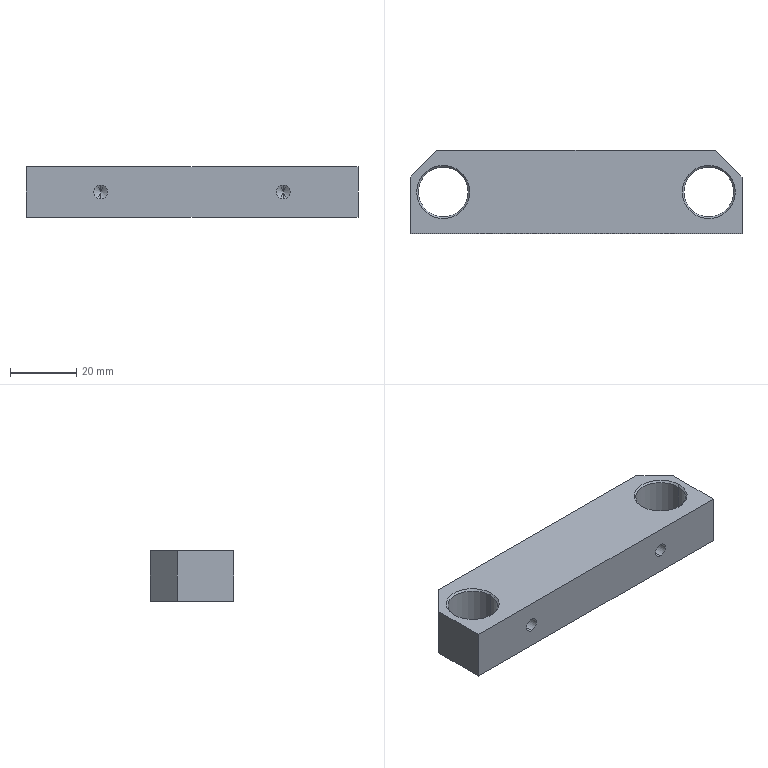Part | STEP file | CA-10-014Pusher Moving Plate_Default | 1 solid | 28 faces | box 100 x 25 x 15.3 mm | volume 31484 mm3 | cone 12 | cylinder 8 | plane 8 | commonest cylinder face diameters 4.2 x4 15 x4